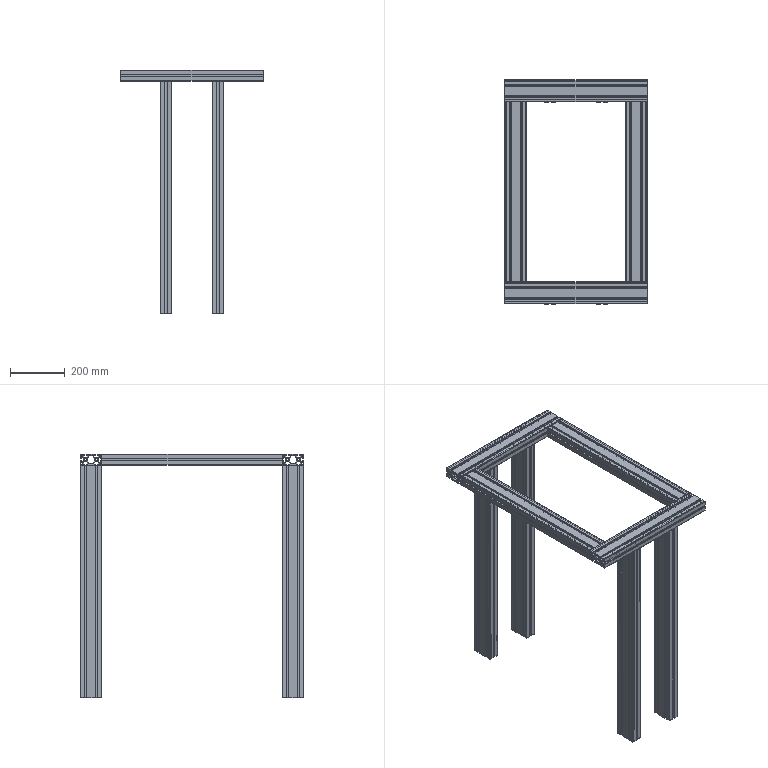Part | STEP file | PN_0009 | 8 solids | 800 faces | box 520 x 820 x 892 mm | volume 7509910 mm3 | plane 480 | cylinder 320 | commonest cylinder face diameters 2 x128 8 x64 19 x64 6 x32 6.8 x32